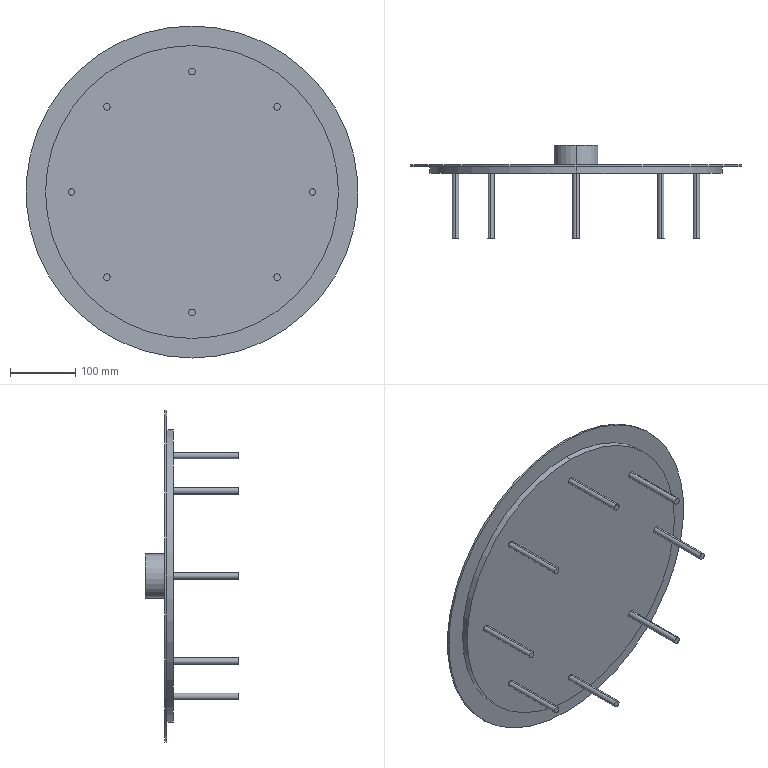Part | SolidWorks | features ICE 3, Extrusion 1 | 1 solid | 34 faces | box 510 x 143 x 510 mm | volume 2374097 mm3 | cylinder 22 | plane 12 | commonest cylinder face diameters 10 x16 67.699 x2 450 x2 510 x2
STEP:
#1=CARTESIAN_POINT('',(0.,43.,33.849));
#2=VERTEX_POINT('',#1);
#3=CARTESIAN_POINT('',(0.,43.,-33.849));
#4=VERTEX_POINT('',#3);
#5=CARTESIAN_POINT('',(0.,43.,0.));
#6=DIRECTION('',(0.,1.,0.));
#7=DIRECTION('',(0.,0.,1.));
#8=AXIS2_PLACEMENT_3D('',#5,#6,#7);
#9=CIRCLE('',#8,33.849);
#10=EDGE_CURVE('',#2,#4,#9,.T.);
#11=ORIENTED_EDGE('',*,*,#10,.F.);
#12=CARTESIAN_POINT('',(0.,13.,33.849));
#13=VERTEX_POINT('',#12);
#14=CARTESIAN_POINT('',(0.,43.,33.849));
#15=DIRECTION('',(0.,-1.,0.));
#16=VECTOR('',#15,1000.);
#17=LINE('',#14,#16);
#18=EDGE_CURVE('',#2,#13,#17,.T.);
#19=ORIENTED_EDGE('',*,*,#18,.T.);
#20=CARTESIAN_POINT('',(0.,13.,-33.849));
#21=VERTEX_POINT('',#20);
#22=CARTESIAN_POINT('',(0.,13.,0.));
#23=DIRECTION('',(0.,1.,0.));
#24=DIRECTION('',(0.,0.,1.));
#25=AXIS2_PLACEMENT_3D('',#22,#23,#24);
#26=CIRCLE('',#25,33.849);
#27=EDGE_CURVE('',#13,#21,#26,.T.);
#28=ORIENTED_EDGE('',*,*,#27,.T.);
#29=CARTESIAN_POINT('',(0.,43.,-33.849));
#30=DIRECTION('',(0.,-1.,0.));
#31=VECTOR('',#30,1000.);
#32=LINE('',#29,#31);
#33=EDGE_CURVE('',#4,#21,#32,.T.);
#34=ORIENTED_EDGE('',*,*,#33,.F.);
#35=EDGE_LOOP('',(#11,#19,#28,#34));
#36=FACE_OUTER_BOUND('',#35,.T.);
#37=CARTESIAN_POINT('',(0.,43.,0.));
#38=DIRECTION('',(0.,-1.,0.));
#39=DIRECTION('',(0.,0.,-1.));
#40=AXIS2_PLACEMENT_3D('',#37,#38,#39);
#41=CYLINDRICAL_SURFACE('',#40,33.849);
#42=ADVANCED_FACE('',(#36),#41,.T.);
#43=CARTESIAN_POINT('',(0.,13.,255.));
#44=VERTEX_POINT('',#43);
#45=CARTESIAN_POINT('',(0.,13.,-255.));
#46=VERTEX_POINT('',#45);
#47=CARTESIAN_POINT('',(0.,13.,0.));
#48=DIRECTION('',(0.,1.,0.));
#49=DIRECTION('',(0.,0.,1.));
#50=AXIS2_PLACEMENT_3D('',#47,#48,#49);
#51=CIRCLE('',#50,255.);
#52=EDGE_CURVE('',#44,#46,#51,.T.);
#53=ORIENTED_EDGE('',*,*,#52,.F.);
#54=CARTESIAN_POINT('',(0.,10.,255.));
#55=VERTEX_POINT('',#54);
#56=CARTESIAN_POINT('',(0.,13.,255.));
#57=DIRECTION('',(0.,-1.,0.));
#58=VECTOR('',#57,1000.);
#59=LINE('',#56,#58);
#60=EDGE_CURVE('',#44,#55,#59,.T.);
#61=ORIENTED_EDGE('',*,*,#60,.T.);
#62=CARTESIAN_POINT('',(0.,10.,-255.));
#63=VERTEX_POINT('',#62);
#64=CARTESIAN_POINT('',(0.,10.,0.));
#65=DIRECTION('',(0.,1.,0.));
#66=DIRECTION('',(0.,0.,1.));
#67=AXIS2_PLACEMENT_3D('',#64,#65,#66);
#68=CIRCLE('',#67,255.);
#69=EDGE_CURVE('',#55,#63,#68,.T.);
#70=ORIENTED_EDGE('',*,*,#69,.T.);
#71=CARTESIAN_POINT('',(0.,13.,-255.));
#72=DIRECTION('',(0.,-1.,0.));
#73=VECTOR('',#72,1000.);
#74=LINE('',#71,#73);
#75=EDGE_CURVE('',#46,#63,#74,.T.);
#76=ORIENTED_EDGE('',*,*,#75,.F.);
#77=EDGE_LOOP('',(#53,#61,#70,#76));
#78=FACE_OUTER_BOUND('',#77,.T.);
#79=CARTESIAN_POINT('',(0.,13.,0.));
#80=DIRECTION('',(0.,-1.,0.));
#81=DIRECTION('',(0.,0.,-1.));
#82=AXIS2_PLACEMENT_3D('',#79,#80,#81);
#83=CYLINDRICAL_SURFACE('',#82,255.);
#84=ADVANCED_FACE('',(#78),#83,.T.);
#85=CARTESIAN_POINT('',(-130.815,-100.,-135.815));
#86=VERTEX_POINT('',#85);
#87=CARTESIAN_POINT('',(-130.815,-100.,-125.815));
#88=VERTEX_POINT('',#87);
#89=CARTESIAN_POINT('',(-130.815,-100.,-130.815));
#90=DIRECTION('',(0.,-1.,0.));
#91=DIRECTION('',(0.,0.,-1.));
#92=AXIS2_PLACEMENT_3D('',#89,#90,#91);
#93=CIRCLE('',#92,5.);
#94=EDGE_CURVE('',#86,#88,#93,.T.);
#95=ORIENTED_EDGE('',*,*,#94,.F.);
#96=CARTESIAN_POINT('',(-130.815,0.,-135.815));
#97=VERTEX_POINT('',#96);
#98=CARTESIAN_POINT('',(-130.815,-100.,-135.815));
#99=DIRECTION('',(0.,1.,0.));
#100=VECTOR('',#99,1000.);
#101=LINE('',#98,#100);
#102=EDGE_CURVE('',#86,#97,#101,.T.);
#103=ORIENTED_EDGE('',*,*,#102,.T.);
#104=CARTESIAN_POINT('',(-130.815,0.,-125.815));
#105=VERTEX_POINT('',#104);
#106=CARTESIAN_POINT('',(-130.815,0.,-130.815));
#107=DIRECTION('',(0.,-1.,0.));
#108=DIRECTION('',(0.,0.,1.));
#109=AXIS2_PLACEMENT_3D('',#106,#107,#108);
#110=CIRCLE('',#109,5.);
#111=EDGE_CURVE('',#97,#105,#110,.T.);
#112=ORIENTED_EDGE('',*,*,#111,.T.);
#113=CARTESIAN_POINT('',(-130.815,-100.,-125.815));
#114=DIRECTION('',(0.,1.,0.));
#115=VECTOR('',#114,1000.);
#116=LINE('',#113,#115);
#117=EDGE_CURVE('',#88,#105,#116,.T.);
#118=ORIENTED_EDGE('',*,*,#117,.F.);
#119=EDGE_LOOP('',(#95,#103,#112,#118));
#120=FACE_OUTER_BOUND('',#119,.T.);
#121=CARTESIAN_POINT('',(-130.815,-100.,-130.815));
#122=DIRECTION('',(0.,1.,0.));
#123=DIRECTION('',(0.,0.,1.));
#124=AXIS2_PLACEMENT_3D('',#121,#122,#123);
#125=CYLINDRICAL_SURFACE('',#124,5.);
#126=ADVANCED_FACE('',(#120),#125,.T.);
#127=CARTESIAN_POINT('',(0.,-100.,-190.));
#128=VERTEX_POINT('',#127);
#129=CARTESIAN_POINT('',(0.,-100.,-180.));
#130=VERTEX_POINT('',#129);
#131=CARTESIAN_POINT('',(0.,-100.,-185.));
#132=DIRECTION('',(0.,-1.,0.));
#133=DIRECTION('',(0.,0.,-1.));
#134=AXIS2_PLACEMENT_3D('',#131,#132,#133);
#135=CIRCLE('',#134,5.);
#136=EDGE_CURVE('',#128,#130,#135,.T.);
#137=ORIENTED_EDGE('',*,*,#136,.F.);
#138=CARTESIAN_POINT('',(0.,0.,-190.));
#139=VERTEX_POINT('',#138);
#140=CARTESIAN_POINT('',(0.,-100.,-190.));
#141=DIRECTION('',(0.,1.,0.));
#142=VECTOR('',#141,1000.);
#143=LINE('',#140,#142);
#144=EDGE_CURVE('',#128,#139,#143,.T.);
#145=ORIENTED_EDGE('',*,*,#144,.T.);
#146=CARTESIAN_POINT('',(0.,0.,-180.));
#147=VERTEX_POINT('',#146);
#148=CARTESIAN_POINT('',(0.,0.,-185.));
#149=DIRECTION('',(0.,-1.,0.));
#150=DIRECTION('',(0.,0.,1.));
#151=AXIS2_PLACEMENT_3D('',#148,#149,#150);
#152=CIRCLE('',#151,5.);
#153=EDGE_CURVE('',#139,#147,#152,.T.);
#154=ORIENTED_EDGE('',*,*,#153,.T.);
#155=CARTESIAN_POINT('',(0.,-100.,-180.));
#156=DIRECTION('',(0.,1.,0.));
#157=VECTOR('',#156,1000.);
#158=LINE('',#155,#157);
#159=EDGE_CURVE('',#130,#147,#158,.T.);
#160=ORIENTED_EDGE('',*,*,#159,.F.);
#161=EDGE_LOOP('',(#137,#145,#154,#160));
#162=FACE_OUTER_BOUND('',#161,.T.);
#163=CARTESIAN_POINT('',(0.,-100.,-185.));
#164=DIRECTION('',(0.,1.,0.));
#165=DIRECTION('',(0.,0.,1.));
#166=AXIS2_PLACEMENT_3D('',#163,#164,#165);
#167=CYLINDRICAL_SURFACE('',#166,5.);
#168=ADVANCED_FACE('',(#162),#167,.T.);
#169=CARTESIAN_POINT('',(130.815,-100.,-135.815));
#170=VERTEX_POINT('',#169);
#171=CARTESIAN_POINT('',(130.815,-100.,-125.815));
#172=VERTEX_POINT('',#171);
#173=CARTESIAN_POINT('',(130.815,-100.,-130.815));
#174=DIRECTION('',(0.,-1.,0.));
#175=DIRECTION('',(0.,0.,-1.));
#176=AXIS2_PLACEMENT_3D('',#173,#174,#175);
#177=CIRCLE('',#176,5.);
#178=EDGE_CURVE('',#170,#172,#177,.T.);
#179=ORIENTED_EDGE('',*,*,#178,.F.);
#180=CARTESIAN_POINT('',(130.815,0.,-135.815));
#181=VERTEX_POINT('',#180);
#182=CARTESIAN_POINT('',(130.815,-100.,-135.815));
#183=DIRECTION('',(0.,1.,0.));
#184=VECTOR('',#183,1000.);
#185=LINE('',#182,#184);
#186=EDGE_CURVE('',#170,#181,#185,.T.);
#187=ORIENTED_EDGE('',*,*,#186,.T.);
#188=CARTESIAN_POINT('',(130.815,0.,-125.815));
#189=VERTEX_POINT('',#188);
#190=CARTESIAN_POINT('',(130.815,0.,-130.815));
#191=DIRECTION('',(0.,-1.,0.));
#192=DIRECTION('',(0.,0.,1.));
#193=AXIS2_PLACEMENT_3D('',#190,#191,#192);
#194=CIRCLE('',#193,5.);
#195=EDGE_CURVE('',#181,#189,#194,.T.);
#196=ORIENTED_EDGE('',*,*,#195,.T.);
#197=CARTESIAN_POINT('',(130.815,-100.,-125.815));
#198=DIRECTION('',(0.,1.,0.));
#199=VECTOR('',#198,1000.);
#200=LINE('',#197,#199);
#201=EDGE_CURVE('',#172,#189,#200,.T.);
#202=ORIENTED_EDGE('',*,*,#201,.F.);
#203=EDGE_LOOP('',(#179,#187,#196,#202));
#204=FACE_OUTER_BOUND('',#203,.T.);
#205=CARTESIAN_POINT('',(130.815,-100.,-130.815));
#206=DIRECTION('',(0.,1.,0.));
#207=DIRECTION('',(0.,0.,1.));
#208=AXIS2_PLACEMENT_3D('',#205,#206,#207);
#209=CYLINDRICAL_SURFACE('',#208,5.);
#210=ADVANCED_FACE('',(#204),#209,.T.);
#211=CARTESIAN_POINT('',(185.,-100.,-5.));
#212=VERTEX_POINT('',#211);
#213=CARTESIAN_POINT('',(185.,-100.,5.));
#214=VERTEX_POINT('',#213);
#215=CARTESIAN_POINT('',(185.,-100.,0.));
#216=DIRECTION('',(0.,-1.,0.));
#217=DIRECTION('',(0.,0.,-1.));
#218=AXIS2_PLACEMENT_3D('',#215,#216,#217);
#219=CIRCLE('',#218,5.);
#220=EDGE_CURVE('',#212,#214,#219,.T.);
#221=ORIENTED_EDGE('',*,*,#220,.F.);
#222=CARTESIAN_POINT('',(185.,0.,-5.));
#223=VERTEX_POINT('',#222);
#224=CARTESIAN_POINT('',(185.,-100.,-5.));
#225=DIRECTION('',(0.,1.,0.));
#226=VECTOR('',#225,1000.);
#227=LINE('',#224,#226);
#228=EDGE_CURVE('',#212,#223,#227,.T.);
#229=ORIENTED_EDGE('',*,*,#228,.T.);
#230=CARTESIAN_POINT('',(185.,0.,5.));
#231=VERTEX_POINT('',#230);
#232=CARTESIAN_POINT('',(185.,0.,0.));
#233=DIRECTION('',(0.,-1.,0.));
#234=DIRECTION('',(0.,0.,1.));
#235=AXIS2_PLACEMENT_3D('',#232,#233,#234);
#236=CIRCLE('',#235,5.);
#237=EDGE_CURVE('',#223,#231,#236,.T.);
#238=ORIENTED_EDGE('',*,*,#237,.T.);
#239=CARTESIAN_POINT('',(185.,-100.,5.));
#240=DIRECTION('',(0.,1.,0.));
#241=VECTOR('',#240,1000.);
#242=LINE('',#239,#241);
#243=EDGE_CURVE('',#214,#231,#242,.T.);
#244=ORIENTED_EDGE('',*,*,#243,.F.);
#245=EDGE_LOOP('',(#221,#229,#238,#244));
#246=FACE_OUTER_BOUND('',#245,.T.);
#247=CARTESIAN_POINT('',(185.,-100.,0.));
#248=DIRECTION('',(0.,1.,0.));
#249=DIRECTION('',(0.,0.,1.));
#250=AXIS2_PLACEMENT_3D('',#247,#248,#249);
#251=CYLINDRICAL_SURFACE('',#250,5.);
#252=ADVANCED_FACE('',(#246),#251,.T.);
#253=CARTESIAN_POINT('',(130.815,-100.,125.815));
#254=VERTEX_POINT('',#253);
#255=CARTESIAN_POINT('',(130.815,-100.,135.815));
#256=VERTEX_POINT('',#255);
#257=CARTESIAN_POINT('',(130.815,-100.,130.815));
#258=DIRECTION('',(0.,-1.,0.));
#259=DIRECTION('',(0.,0.,-1.));
#260=AXIS2_PLACEMENT_3D('',#257,#258,#259);
#261=CIRCLE('',#260,5.);
#262=EDGE_CURVE('',#254,#256,#261,.T.);
#263=ORIENTED_EDGE('',*,*,#262,.F.);
#264=CARTESIAN_POINT('',(130.815,0.,125.815));
#265=VERTEX_POINT('',#264);
#266=CARTESIAN_POINT('',(130.815,-100.,125.815));
#267=DIRECTION('',(0.,1.,0.));
#268=VECTOR('',#267,1000.);
#269=LINE('',#266,#268);
#270=EDGE_CURVE('',#254,#265,#269,.T.);
#271=ORIENTED_EDGE('',*,*,#270,.T.);
#272=CARTESIAN_POINT('',(130.815,0.,135.815));
#273=VERTEX_POINT('',#272);
#274=CARTESIAN_POINT('',(130.815,0.,130.815));
#275=DIRECTION('',(0.,-1.,0.));
#276=DIRECTION('',(0.,0.,1.));
#277=AXIS2_PLACEMENT_3D('',#274,#275,#276);
#278=CIRCLE('',#277,5.);
#279=EDGE_CURVE('',#265,#273,#278,.T.);
#280=ORIENTED_EDGE('',*,*,#279,.T.);
#281=CARTESIAN_POINT('',(130.815,-100.,135.815));
#282=DIRECTION('',(0.,1.,0.));
#283=VECTOR('',#282,1000.);
#284=LINE('',#281,#283);
#285=EDGE_CURVE('',#256,#273,#284,.T.);
#286=ORIENTED_EDGE('',*,*,#285,.F.);
#287=EDGE_LOOP('',(#263,#271,#280,#286));
#288=FACE_OUTER_BOUND('',#287,.T.);
#289=CARTESIAN_POINT('',(130.815,-100.,130.815));
#290=DIRECTION('',(0.,1.,0.));
#291=DIRECTION('',(0.,0.,1.));
#292=AXIS2_PLACEMENT_3D('',#289,#290,#291);
#293=CYLINDRICAL_SURFACE('',#292,5.);
#294=ADVANCED_FACE('',(#288),#293,.T.);
#295=CARTESIAN_POINT('',(0.,-100.,180.));
#296=VERTEX_POINT('',#295);
#297=CARTESIAN_POINT('',(0.,-100.,190.));
#298=VERTEX_POINT('',#297);
#299=CARTESIAN_POINT('',(0.,-100.,185.));
#300=DIRECTION('',(0.,-1.,0.));
#301=DIRECTION('',(0.,0.,-1.));
#302=AXIS2_PLACEMENT_3D('',#299,#300,#301);
#303=CIRCLE('',#302,5.);
#304=EDGE_CURVE('',#296,#298,#303,.T.);
#305=ORIENTED_EDGE('',*,*,#304,.F.);
#306=CARTESIAN_POINT('',(0.,0.,180.));
#307=VERTEX_POINT('',#306);
#308=CARTESIAN_POINT('',(0.,-100.,180.));
#309=DIRECTION('',(0.,1.,0.));
#310=VECTOR('',#309,1000.);
#311=LINE('',#308,#310);
#312=EDGE_CURVE('',#296,#307,#311,.T.);
#313=ORIENTED_EDGE('',*,*,#312,.T.);
#314=CARTESIAN_POINT('',(0.,0.,190.));
#315=VERTEX_POINT('',#314);
#316=CARTESIAN_POINT('',(0.,0.,185.));
#317=DIRECTION('',(0.,-1.,0.));
#318=DIRECTION('',(0.,0.,1.));
#319=AXIS2_PLACEMENT_3D('',#316,#317,#318);
#320=CIRCLE('',#319,5.);
#321=EDGE_CURVE('',#307,#315,#320,.T.);
#322=ORIENTED_EDGE('',*,*,#321,.T.);
#323=CARTESIAN_POINT('',(0.,-100.,190.));
#324=DIRECTION('',(0.,1.,0.));
#325=VECTOR('',#324,1000.);
#326=LINE('',#323,#325);
#327=EDGE_CURVE('',#298,#315,#326,.T.);
#328=ORIENTED_EDGE('',*,*,#327,.F.);
#329=EDGE_LOOP('',(#305,#313,#322,#328));
#330=FACE_OUTER_BOUND('',#329,.T.);
#331=CARTESIAN_POINT('',(0.,-100.,185.));
#332=DIRECTION('',(0.,1.,0.));
#333=DIRECTION('',(0.,0.,1.));
#334=AXIS2_PLACEMENT_3D('',#331,#332,#333);
#335=CYLINDRICAL_SURFACE('',#334,5.);
#336=ADVANCED_FACE('',(#330),#335,.T.);
#337=CARTESIAN_POINT('',(-130.815,-100.,125.815));
#338=VERTEX_POINT('',#337);
#339=CARTESIAN_POINT('',(-130.815,-100.,135.815));
#340=VERTEX_POINT('',#339);
#341=CARTESIAN_POINT('',(-130.815,-100.,130.815));
#342=DIRECTION('',(0.,-1.,0.));
#343=DIRECTION('',(0.,0.,-1.));
#344=AXIS2_PLACEMENT_3D('',#341,#342,#343);
#345=CIRCLE('',#344,5.);
#346=EDGE_CURVE('',#338,#340,#345,.T.);
#347=ORIENTED_EDGE('',*,*,#346,.F.);
#348=CARTESIAN_POINT('',(-130.815,0.,125.815));
#349=VERTEX_POINT('',#348);
#350=CARTESIAN_POINT('',(-130.815,-100.,125.815));
#351=DIRECTION('',(0.,1.,0.));
#352=VECTOR('',#351,1000.);
#353=LINE('',#350,#352);
#354=EDGE_CURVE('',#338,#349,#353,.T.);
#355=ORIENTED_EDGE('',*,*,#354,.T.);
#356=CARTESIAN_POINT('',(-130.815,0.,135.815));
#357=VERTEX_POINT('',#356);
#358=CARTESIAN_POINT('',(-130.815,0.,130.815));
#359=DIRECTION('',(0.,-1.,0.));
#360=DIRECTION('',(0.,0.,1.));
#361=AXIS2_PLACEMENT_3D('',#358,#359,#360);
#362=CIRCLE('',#361,5.);
#363=EDGE_CURVE('',#349,#357,#362,.T.);
#364=ORIENTED_EDGE('',*,*,#363,.T.);
#365=CARTESIAN_POINT('',(-130.815,-100.,135.815));
#366=DIRECTION('',(0.,1.,0.));
#367=VECTOR('',#366,1000.);
#368=LINE('',#365,#367);
#369=EDGE_CURVE('',#340,#357,#368,.T.);
#370=ORIENTED_EDGE('',*,*,#369,.F.);
#371=EDGE_LOOP('',(#347,#355,#364,#370));
#372=FACE_OUTER_BOUND('',#371,.T.);
#373=CARTESIAN_POINT('',(-130.815,-100.,130.815));
#374=DIRECTION('',(0.,1.,0.));
#375=DIRECTION('',(0.,0.,1.));
#376=AXIS2_PLACEMENT_3D('',#373,#374,#375);
#377=CYLINDRICAL_SURFACE('',#376,5.);
#378=ADVANCED_FACE('',(#372),#377,.T.);
#379=CARTESIAN_POINT('',(-185.,-100.,-5.));
#380=VERTEX_POINT('',#379);
#381=CARTESIAN_POINT('',(-185.,-100.,5.));
#382=VERTEX_POINT('',#381);
#383=CARTESIAN_POINT('',(-185.,-100.,0.));
#384=DIRECTION('',(0.,-1.,0.));
#385=DIRECTION('',(0.,0.,-1.));
#386=AXIS2_PLACEMENT_3D('',#383,#384,#385);
#387=CIRCLE('',#386,5.);
#388=EDGE_CURVE('',#380,#382,#387,.T.);
#389=ORIENTED_EDGE('',*,*,#388,.F.);
#390=CARTESIAN_POINT('',(-185.,0.,-5.));
#391=VERTEX_POINT('',#390);
#392=CARTESIAN_POINT('',(-185.,-100.,-5.));
#393=DIRECTION('',(0.,1.,0.));
#394=VECTOR('',#393,1000.);
#395=LINE('',#392,#394);
#396=EDGE_CURVE('',#380,#391,#395,.T.);
#397=ORIENTED_EDGE('',*,*,#396,.T.);
#398=CARTESIAN_POINT('',(-185.,0.,5.));
#399=VERTEX_POINT('',#398);
#400=CARTESIAN_POINT('',(-185.,0.,0.));
#401=DIRECTION('',(0.,-1.,0.));
#402=DIRECTION('',(0.,0.,1.));
#403=AXIS2_PLACEMENT_3D('',#400,#401,#402);
#404=CIRCLE('',#403,5.);
#405=EDGE_CURVE('',#391,#399,#404,.T.);
#406=ORIENTED_EDGE('',*,*,#405,.T.);
#407=CARTESIAN_POINT('',(-185.,-100.,5.));
#408=DIRECTION('',(0.,1.,0.));
#409=VECTOR('',#408,1000.);
#410=LINE('',#407,#409);
#411=EDGE_CURVE('',#382,#399,#410,.T.);
#412=ORIENTED_EDGE('',*,*,#411,.F.);
#413=EDGE_LOOP('',(#389,#397,#406,#412));
#414=FACE_OUTER_BOUND('',#413,.T.);
#415=CARTESIAN_POINT('',(-185.,-100.,0.));
#416=DIRECTION('',(0.,1.,0.));
#417=DIRECTION('',(0.,0.,1.));
#418=AXIS2_PLACEMENT_3D('',#415,#416,#417);
#419=CYLINDRICAL_SURFACE('',#418,5.);
#420=ADVANCED_FACE('',(#414),#419,.T.);
#421=CARTESIAN_POINT('',(0.,10.,225.));
#422=VERTEX_POINT('',#421);
#423=CARTESIAN_POINT('',(0.,10.,-225.));
#424=VERTEX_POINT('',#423);
#425=CARTESIAN_POINT('',(0.,10.,0.));
#426=DIRECTION('',(0.,1.,0.));
#427=DIRECTION('',(0.,0.,1.));
#428=AXIS2_PLACEMENT_3D('',#425,#426,#427);
#429=CIRCLE('',#428,225.);
#430=EDGE_CURVE('',#422,#424,#429,.T.);
#431=ORIENTED_EDGE('',*,*,#430,.F.);
#432=CARTESIAN_POINT('',(0.,0.,225.));
#433=VERTEX_POINT('',#432);
#434=CARTESIAN_POINT('',(0.,10.,225.));
#435=DIRECTION('',(0.,-1.,0.));
#436=VECTOR('',#435,1000.);
#437=LINE('',#434,#436);
#438=EDGE_CURVE('',#422,#433,#437,.T.);
#439=ORIENTED_EDGE('',*,*,#438,.T.);
#440=CARTESIAN_POINT('',(0.,0.,-225.));
#441=VERTEX_POINT('',#440);
#442=CARTESIAN_POINT('',(0.,0.,0.));
#443=DIRECTION('',(0.,1.,0.));
#444=DIRECTION('',(0.,0.,1.));
#445=AXIS2_PLACEMENT_3D('',#442,#443,#444);
#446=CIRCLE('',#445,225.);
#447=EDGE_CURVE('',#433,#441,#446,.T.);
#448=ORIENTED_EDGE('',*,*,#447,.T.);
#449=CARTESIAN_POINT('',(0.,10.,-225.));
#450=DIRECTION('',(0.,-1.,0.));
#451=VECTOR('',#450,1000.);
#452=LINE('',#449,#451);
#453=EDGE_CURVE('',#424,#441,#452,.T.);
#454=ORIENTED_EDGE('',*,*,#453,.F.);
#455=EDGE_LOOP('',(#431,#439,#448,#454));
#456=FACE_OUTER_BOUND('',#455,.T.);
#457=CARTESIAN_POINT('',(0.,10.,0.));
#458=DIRECTION('',(0.,-1.,0.));
#459=DIRECTION('',(0.,0.,-1.));
#460=AXIS2_PLACEMENT_3D('',#457,#458,#459);
#461=CYLINDRICAL_SURFACE('',#460,225.);
#462=ADVANCED_FACE('',(#456),#461,.T.);
#463=ORIENTED_EDGE('',*,*,#438,.F.);
#464=CARTESIAN_POINT('',(0.,10.,0.));
#465=DIRECTION('',(0.,1.,0.));
#466=DIRECTION('',(0.,0.,1.));
#467=AXIS2_PLACEMENT_3D('',#464,#465,#466);
#468=CIRCLE('',#467,225.);
#469=EDGE_CURVE('',#424,#422,#468,.T.);
#470=ORIENTED_EDGE('',*,*,#469,.F.);
#471=ORIENTED_EDGE('',*,*,#453,.T.);
#472=CARTESIAN_POINT('',(0.,0.,0.));
#473=DIRECTION('',(0.,1.,0.));
#474=DIRECTION('',(0.,0.,1.));
#475=AXIS2_PLACEMENT_3D('',#472,#473,#474);
#476=CIRCLE('',#475,225.);
#477=EDGE_CURVE('',#441,#433,#476,.T.);
#478=ORIENTED_EDGE('',*,*,#477,.T.);
#479=EDGE_LOOP('',(#463,#470,#471,#478));
#480=FACE_OUTER_BOUND('',#479,.T.);
#481=CARTESIAN_POINT('',(0.,10.,0.));
#482=DIRECTION('',(0.,-1.,0.));
#483=DIRECTION('',(0.,0.,-1.));
#484=AXIS2_PLACEMENT_3D('',#481,#482,#483);
#485=CYLINDRICAL_SURFACE('',#484,225.);
#486=ADVANCED_FACE('',(#480),#485,.T.);
#487=CARTESIAN_POINT('',(-130.815,0.,-130.815));
#488=DIRECTION('',(0.,-1.,0.));
#489=DIRECTION('',(0.,0.,1.));
#490=AXIS2_PLACEMENT_3D('',#487,#488,#489);
#491=CIRCLE('',#490,5.);
#492=EDGE_CURVE('',#105,#97,#491,.T.);
#493=ORIENTED_EDGE('',*,*,#492,.F.);
#494=ORIENTED_EDGE('',*,*,#111,.F.);
#495=EDGE_LOOP('',(#493,#494));
#496=FACE_BOUND('',#495,.T.);
#497=CARTESIAN_POINT('',(0.,0.,-185.));
#498=DIRECTION('',(0.,-1.,0.));
#499=DIRECTION('',(0.,0.,1.));
#500=AXIS2_PLACEMENT_3D('',#497,#498,#499);
#501=CIRCLE('',#500,5.);
#502=EDGE_CURVE('',#147,#139,#501,.T.);
#503=ORIENTED_EDGE('',*,*,#502,.F.);
#504=ORIENTED_EDGE('',*,*,#153,.F.);
#505=EDGE_LOOP('',(#503,#504));
#506=FACE_BOUND('',#505,.T.);
#507=CARTESIAN_POINT('',(130.815,0.,-130.815));
#508=DIRECTION('',(0.,-1.,0.));
#509=DIRECTION('',(0.,0.,1.));
#510=AXIS2_PLACEMENT_3D('',#507,#508,#509);
#511=CIRCLE('',#510,5.);
#512=EDGE_CURVE('',#189,#181,#511,.T.);
#513=ORIENTED_EDGE('',*,*,#512,.F.);
#514=ORIENTED_EDGE('',*,*,#195,.F.);
#515=EDGE_LOOP('',(#513,#514));
#516=FACE_BOUND('',#515,.T.);
#517=CARTESIAN_POINT('',(185.,0.,0.));
#518=DIRECTION('',(0.,-1.,0.));
#519=DIRECTION('',(0.,0.,1.));
#520=AXIS2_PLACEMENT_3D('',#517,#518,#519);
#521=CIRCLE('',#520,5.);
#522=EDGE_CURVE('',#231,#223,#521,.T.);
#523=ORIENTED_EDGE('',*,*,#522,.F.);
#524=ORIENTED_EDGE('',*,*,#237,.F.);
#525=EDGE_LOOP('',(#523,#524));
#526=FACE_BOUND('',#525,.T.);
#527=CARTESIAN_POINT('',(130.815,0.,130.815));
#528=DIRECTION('',(0.,-1.,0.));
#529=DIRECTION('',(0.,0.,1.));
#530=AXIS2_PLACEMENT_3D('',#527,#528,#529);
#531=CIRCLE('',#530,5.);
#532=EDGE_CURVE('',#273,#265,#531,.T.);
#533=ORIENTED_EDGE('',*,*,#532,.F.);
#534=ORIENTED_EDGE('',*,*,#279,.F.);
#535=EDGE_LOOP('',(#533,#534));
#536=FACE_BOUND('',#535,.T.);
#537=CARTESIAN_POINT('',(0.,0.,185.));
#538=DIRECTION('',(0.,-1.,0.));
#539=DIRECTION('',(0.,0.,1.));
#540=AXIS2_PLACEMENT_3D('',#537,#538,#539);
#541=CIRCLE('',#540,5.);
#542=EDGE_CURVE('',#315,#307,#541,.T.);
#543=ORIENTED_EDGE('',*,*,#542,.F.);
#544=ORIENTED_EDGE('',*,*,#321,.F.);
#545=EDGE_LOOP('',(#543,#544));
#546=FACE_BOUND('',#545,.T.);
#547=CARTESIAN_POINT('',(-130.815,0.,130.815));
#548=DIRECTION('',(0.,-1.,0.));
#549=DIRECTION('',(0.,0.,1.));
#550=AXIS2_PLACEMENT_3D('',#547,#548,#549);
#551=CIRCLE('',#550,5.);
#552=EDGE_CURVE('',#357,#349,#551,.T.);
#553=ORIENTED_EDGE('',*,*,#552,.F.);
#554=ORIENTED_EDGE('',*,*,#363,.F.);
#555=EDGE_LOOP('',(#553,#554));
#556=FACE_BOUND('',#555,.T.);
#557=CARTESIAN_POINT('',(-185.,0.,0.));
#558=DIRECTION('',(0.,-1.,0.));
#559=DIRECTION('',(0.,0.,1.));
#560=AXIS2_PLACEMENT_3D('',#557,#558,#559);
#561=CIRCLE('',#560,5.);
#562=EDGE_CURVE('',#399,#391,#561,.T.);
#563=ORIENTED_EDGE('',*,*,#562,.F.);
#564=ORIENTED_EDGE('',*,*,#405,.F.);
#565=EDGE_LOOP('',(#563,#564));
#566=FACE_BOUND('',#565,.T.);
#567=ORIENTED_EDGE('',*,*,#477,.F.);
#568=ORIENTED_EDGE('',*,*,#447,.F.);
#569=EDGE_LOOP('',(#567,#568));
#570=FACE_OUTER_BOUND('',#569,.T.);
#571=CARTESIAN_POINT('',(0.,0.,0.));
#572=DIRECTION('',(0.,1.,0.));
#573=DIRECTION('',(0.,0.,1.));
#574=AXIS2_PLACEMENT_3D('',#571,#572,#573);
#575=PLANE('',#574);
#576=ADVANCED_FACE('',(#496,#506,#516,#526,#536,#546,#556,#566,#570),#575,.F.);
#577=ORIENTED_EDGE('',*,*,#396,.F.);
#578=CARTESIAN_POINT('',(-185.,-100.,0.));
#579=DIRECTION('',(0.,-1.,0.));
#580=DIRECTION('',(0.,0.,-1.));
#581=AXIS2_PLACEMENT_3D('',#578,#579,#580);
#582=CIRCLE('',#581,5.);
#583=EDGE_CURVE('',#382,#380,#582,.T.);
#584=ORIENTED_EDGE('',*,*,#583,.F.);
#585=ORIENTED_EDGE('',*,*,#411,.T.);
#586=ORIENTED_EDGE('',*,*,#562,.T.);
#587=EDGE_LOOP('',(#577,#584,#585,#586));
#588=FACE_OUTER_BOUND('',#587,.T.);
#589=CARTESIAN_POINT('',(-185.,-100.,0.));
#590=DIRECTION('',(0.,1.,0.));
#591=DIRECTION('',(0.,0.,1.));
#592=AXIS2_PLACEMENT_3D('',#589,#590,#591);
#593=CYLINDRICAL_SURFACE('',#592,5.);
#594=ADVANCED_FACE('',(#588),#593,.T.);
#595=ORIENTED_EDGE('',*,*,#583,.T.);
#596=ORIENTED_EDGE('',*,*,#388,.T.);
#597=EDGE_LOOP('',(#595,#596));
#598=FACE_OUTER_BOUND('',#597,.T.);
#599=CARTESIAN_POINT('',(-185.,-100.,0.));
#600=DIRECTION('',(0.,-1.,0.));
#601=DIRECTION('',(0.,0.,-1.));
#602=AXIS2_PLACEMENT_3D('',#599,#600,#601);
#603=PLANE('',#602);
#604=ADVANCED_FACE('',(#598),#603,.T.);
#605=ORIENTED_EDGE('',*,*,#354,.F.);
#606=CARTESIAN_POINT('',(-130.815,-100.,130.815));
#607=DIRECTION('',(0.,-1.,0.));
#608=DIRECTION('',(0.,0.,-1.));
#609=AXIS2_PLACEMENT_3D('',#606,#607,#608);
#610=CIRCLE('',#609,5.);
#611=EDGE_CURVE('',#340,#338,#610,.T.);
#612=ORIENTED_EDGE('',*,*,#611,.F.);
#613=ORIENTED_EDGE('',*,*,#369,.T.);
#614=ORIENTED_EDGE('',*,*,#552,.T.);
#615=EDGE_LOOP('',(#605,#612,#613,#614));
#616=FACE_OUTER_BOUND('',#615,.T.);
#617=CARTESIAN_POINT('',(-130.815,-100.,130.815));
#618=DIRECTION('',(0.,1.,0.));
#619=DIRECTION('',(0.,0.,1.));
#620=AXIS2_PLACEMENT_3D('',#617,#618,#619);
#621=CYLINDRICAL_SURFACE('',#620,5.);
#622=ADVANCED_FACE('',(#616),#621,.T.);
#623=ORIENTED_EDGE('',*,*,#611,.T.);
#624=ORIENTED_EDGE('',*,*,#346,.T.);
#625=EDGE_LOOP('',(#623,#624));
#626=FACE_OUTER_BOUND('',#625,.T.);
#627=CARTESIAN_POINT('',(-130.815,-100.,130.815));
#628=DIRECTION('',(0.,-1.,0.));
#629=DIRECTION('',(0.,0.,-1.));
#630=AXIS2_PLACEMENT_3D('',#627,#628,#629);
#631=PLANE('',#630);
#632=ADVANCED_FACE('',(#626),#631,.T.);
#633=ORIENTED_EDGE('',*,*,#312,.F.);
#634=CARTESIAN_POINT('',(0.,-100.,185.));
#635=DIRECTION('',(0.,-1.,0.));
#636=DIRECTION('',(0.,0.,-1.));
#637=AXIS2_PLACEMENT_3D('',#634,#635,#636);
#638=CIRCLE('',#637,5.);
#639=EDGE_CURVE('',#298,#296,#638,.T.);
#640=ORIENTED_EDGE('',*,*,#639,.F.);
#641=ORIENTED_EDGE('',*,*,#327,.T.);
#642=ORIENTED_EDGE('',*,*,#542,.T.);
#643=EDGE_LOOP('',(#633,#640,#641,#642));
#644=FACE_OUTER_BOUND('',#643,.T.);
#645=CARTESIAN_POINT('',(0.,-100.,185.));
#646=DIRECTION('',(0.,1.,0.));
#647=DIRECTION('',(0.,0.,1.));
#648=AXIS2_PLACEMENT_3D('',#645,#646,#647);
#649=CYLINDRICAL_SURFACE('',#648,5.);
#650=ADVANCED_FACE('',(#644),#649,.T.);
#651=ORIENTED_EDGE('',*,*,#639,.T.);
#652=ORIENTED_EDGE('',*,*,#304,.T.);
#653=EDGE_LOOP('',(#651,#652));
#654=FACE_OUTER_BOUND('',#653,.T.);
#655=CARTESIAN_POINT('',(0.,-100.,185.));
#656=DIRECTION('',(0.,-1.,0.));
#657=DIRECTION('',(0.,0.,-1.));
#658=AXIS2_PLACEMENT_3D('',#655,#656,#657);
#659=PLANE('',#658);
#660=ADVANCED_FACE('',(#654),#659,.T.);
#661=ORIENTED_EDGE('',*,*,#270,.F.);
#662=CARTESIAN_POINT('',(130.815,-100.,130.815));
#663=DIRECTION('',(0.,-1.,0.));
#664=DIRECTION('',(0.,0.,-1.));
#665=AXIS2_PLACEMENT_3D('',#662,#663,#664);
#666=CIRCLE('',#665,5.);
#667=EDGE_CURVE('',#256,#254,#666,.T.);
#668=ORIENTED_EDGE('',*,*,#667,.F.);
#669=ORIENTED_EDGE('',*,*,#285,.T.);
#670=ORIENTED_EDGE('',*,*,#532,.T.);
#671=EDGE_LOOP('',(#661,#668,#669,#670));
#672=FACE_OUTER_BOUND('',#671,.T.);
#673=CARTESIAN_POINT('',(130.815,-100.,130.815));
#674=DIRECTION('',(0.,1.,0.));
#675=DIRECTION('',(0.,0.,1.));
#676=AXIS2_PLACEMENT_3D('',#673,#674,#675);
#677=CYLINDRICAL_SURFACE('',#676,5.);
#678=ADVANCED_FACE('',(#672),#677,.T.);
#679=ORIENTED_EDGE('',*,*,#667,.T.);
#680=ORIENTED_EDGE('',*,*,#262,.T.);
#681=EDGE_LOOP('',(#679,#680));
#682=FACE_OUTER_BOUND('',#681,.T.);
#683=CARTESIAN_POINT('',(130.815,-100.,130.815));
#684=DIRECTION('',(0.,-1.,0.));
#685=DIRECTION('',(0.,0.,-1.));
#686=AXIS2_PLACEMENT_3D('',#683,#684,#685);
#687=PLANE('',#686);
#688=ADVANCED_FACE('',(#682),#687,.T.);
#689=ORIENTED_EDGE('',*,*,#228,.F.);
#690=CARTESIAN_POINT('',(185.,-100.,0.));
#691=DIRECTION('',(0.,-1.,0.));
#692=DIRECTION('',(0.,0.,-1.));
#693=AXIS2_PLACEMENT_3D('',#690,#691,#692);
#694=CIRCLE('',#693,5.);
#695=EDGE_CURVE('',#214,#212,#694,.T.);
#696=ORIENTED_EDGE('',*,*,#695,.F.);
#697=ORIENTED_EDGE('',*,*,#243,.T.);
#698=ORIENTED_EDGE('',*,*,#522,.T.);
#699=EDGE_LOOP('',(#689,#696,#697,#698));
#700=FACE_OUTER_BOUND('',#699,.T.);
#701=CARTESIAN_POINT('',(185.,-100.,0.));
#702=DIRECTION('',(0.,1.,0.));
#703=DIRECTION('',(0.,0.,1.));
#704=AXIS2_PLACEMENT_3D('',#701,#702,#703);
#705=CYLINDRICAL_SURFACE('',#704,5.);
#706=ADVANCED_FACE('',(#700),#705,.T.);
#707=ORIENTED_EDGE('',*,*,#695,.T.);
#708=ORIENTED_EDGE('',*,*,#220,.T.);
#709=EDGE_LOOP('',(#707,#708));
#710=FACE_OUTER_BOUND('',#709,.T.);
#711=CARTESIAN_POINT('',(185.,-100.,0.));
#712=DIRECTION('',(0.,-1.,0.));
#713=DIRECTION('',(0.,0.,-1.));
#714=AXIS2_PLACEMENT_3D('',#711,#712,#713);
#715=PLANE('',#714);
#716=ADVANCED_FACE('',(#710),#715,.T.);
#717=ORIENTED_EDGE('',*,*,#186,.F.);
#718=CARTESIAN_POINT('',(130.815,-100.,-130.815));
#719=DIRECTION('',(0.,-1.,0.));
#720=DIRECTION('',(0.,0.,-1.));
#721=AXIS2_PLACEMENT_3D('',#718,#719,#720);
#722=CIRCLE('',#721,5.);
#723=EDGE_CURVE('',#172,#170,#722,.T.);
#724=ORIENTED_EDGE('',*,*,#723,.F.);
#725=ORIENTED_EDGE('',*,*,#201,.T.);
#726=ORIENTED_EDGE('',*,*,#512,.T.);
#727=EDGE_LOOP('',(#717,#724,#725,#726));
#728=FACE_OUTER_BOUND('',#727,.T.);
#729=CARTESIAN_POINT('',(130.815,-100.,-130.815));
#730=DIRECTION('',(0.,1.,0.));
#731=DIRECTION('',(0.,0.,1.));
#732=AXIS2_PLACEMENT_3D('',#729,#730,#731);
#733=CYLINDRICAL_SURFACE('',#732,5.);
#734=ADVANCED_FACE('',(#728),#733,.T.);
#735=ORIENTED_EDGE('',*,*,#723,.T.);
#736=ORIENTED_EDGE('',*,*,#178,.T.);
#737=EDGE_LOOP('',(#735,#736));
#738=FACE_OUTER_BOUND('',#737,.T.);
#739=CARTESIAN_POINT('',(130.815,-100.,-130.815));
#740=DIRECTION('',(0.,-1.,0.));
#741=DIRECTION('',(0.,0.,-1.));
#742=AXIS2_PLACEMENT_3D('',#739,#740,#741);
#743=PLANE('',#742);
#744=ADVANCED_FACE('',(#738),#743,.T.);
#745=ORIENTED_EDGE('',*,*,#144,.F.);
#746=CARTESIAN_POINT('',(0.,-100.,-185.));
#747=DIRECTION('',(0.,-1.,0.));
#748=DIRECTION('',(0.,0.,-1.));
#749=AXIS2_PLACEMENT_3D('',#746,#747,#748);
#750=CIRCLE('',#749,5.);
#751=EDGE_CURVE('',#130,#128,#750,.T.);
#752=ORIENTED_EDGE('',*,*,#751,.F.);
#753=ORIENTED_EDGE('',*,*,#159,.T.);
#754=ORIENTED_EDGE('',*,*,#502,.T.);
#755=EDGE_LOOP('',(#745,#752,#753,#754));
#756=FACE_OUTER_BOUND('',#755,.T.);
#757=CARTESIAN_POINT('',(0.,-100.,-185.));
#758=DIRECTION('',(0.,1.,0.));
#759=DIRECTION('',(0.,0.,1.));
#760=AXIS2_PLACEMENT_3D('',#757,#758,#759);
#761=CYLINDRICAL_SURFACE('',#760,5.);
#762=ADVANCED_FACE('',(#756),#761,.T.);
#763=ORIENTED_EDGE('',*,*,#751,.T.);
#764=ORIENTED_EDGE('',*,*,#136,.T.);
#765=EDGE_LOOP('',(#763,#764));
#766=FACE_OUTER_BOUND('',#765,.T.);
#767=CARTESIAN_POINT('',(0.,-100.,-185.));
#768=DIRECTION('',(0.,-1.,0.));
#769=DIRECTION('',(0.,0.,-1.));
#770=AXIS2_PLACEMENT_3D('',#767,#768,#769);
#771=PLANE('',#770);
#772=ADVANCED_FACE('',(#766),#771,.T.);
#773=ORIENTED_EDGE('',*,*,#102,.F.);
#774=CARTESIAN_POINT('',(-130.815,-100.,-130.815));
#775=DIRECTION('',(0.,-1.,0.));
#776=DIRECTION('',(0.,0.,-1.));
#777=AXIS2_PLACEMENT_3D('',#774,#775,#776);
#778=CIRCLE('',#777,5.);
#779=EDGE_CURVE('',#88,#86,#778,.T.);
#780=ORIENTED_EDGE('',*,*,#779,.F.);
#781=ORIENTED_EDGE('',*,*,#117,.T.);
#782=ORIENTED_EDGE('',*,*,#492,.T.);
#783=EDGE_LOOP('',(#773,#780,#781,#782));
#784=FACE_OUTER_BOUND('',#783,.T.);
#785=CARTESIAN_POINT('',(-130.815,-100.,-130.815));
#786=DIRECTION('',(0.,1.,0.));
#787=DIRECTION('',(0.,0.,1.));
#788=AXIS2_PLACEMENT_3D('',#785,#786,#787);
#789=CYLINDRICAL_SURFACE('',#788,5.);
#790=ADVANCED_FACE('',(#784),#789,.T.);
#791=ORIENTED_EDGE('',*,*,#779,.T.);
#792=ORIENTED_EDGE('',*,*,#94,.T.);
#793=EDGE_LOOP('',(#791,#792));
#794=FACE_OUTER_BOUND('',#793,.T.);
#795=CARTESIAN_POINT('',(-130.815,-100.,-130.815));
#796=DIRECTION('',(0.,-1.,0.));
#797=DIRECTION('',(0.,0.,-1.));
#798=AXIS2_PLACEMENT_3D('',#795,#796,#797);
#799=PLANE('',#798);
#800=ADVANCED_FACE('',(#794),#799,.T.);
#801=ORIENTED_EDGE('',*,*,#60,.F.);
#802=CARTESIAN_POINT('',(0.,13.,0.));
#803=DIRECTION('',(0.,1.,0.));
#804=DIRECTION('',(0.,0.,1.));
#805=AXIS2_PLACEMENT_3D('',#802,#803,#804);
#806=CIRCLE('',#805,255.);
#807=EDGE_CURVE('',#46,#44,#806,.T.);
#808=ORIENTED_EDGE('',*,*,#807,.F.);
#809=ORIENTED_EDGE('',*,*,#75,.T.);
#810=CARTESIAN_POINT('',(0.,10.,0.));
#811=DIRECTION('',(0.,1.,0.));
#812=DIRECTION('',(0.,0.,1.));
#813=AXIS2_PLACEMENT_3D('',#810,#811,#812);
#814=CIRCLE('',#813,255.);
#815=EDGE_CURVE('',#63,#55,#814,.T.);
#816=ORIENTED_EDGE('',*,*,#815,.T.);
#817=EDGE_LOOP('',(#801,#808,#809,#816));
#818=FACE_OUTER_BOUND('',#817,.T.);
#819=CARTESIAN_POINT('',(0.,13.,0.));
#820=DIRECTION('',(0.,-1.,0.));
#821=DIRECTION('',(0.,0.,-1.));
#822=AXIS2_PLACEMENT_3D('',#819,#820,#821);
#823=CYLINDRICAL_SURFACE('',#822,255.);
#824=ADVANCED_FACE('',(#818),#823,.T.);
#825=CARTESIAN_POINT('',(0.,13.,0.));
#826=DIRECTION('',(0.,1.,0.));
#827=DIRECTION('',(0.,0.,1.));
#828=AXIS2_PLACEMENT_3D('',#825,#826,#827);
#829=CIRCLE('',#828,33.849);
#830=EDGE_CURVE('',#21,#13,#829,.T.);
#831=ORIENTED_EDGE('',*,*,#830,.F.);
#832=ORIENTED_EDGE('',*,*,#27,.F.);
#833=EDGE_LOOP('',(#831,#832));
#834=FACE_BOUND('',#833,.T.);
#835=ORIENTED_EDGE('',*,*,#807,.T.);
#836=ORIENTED_EDGE('',*,*,#52,.T.);
#837=EDGE_LOOP('',(#835,#836));
#838=FACE_OUTER_BOUND('',#837,.T.);
#839=CARTESIAN_POINT('',(0.,13.,0.));
#840=DIRECTION('',(0.,1.,0.));
#841=DIRECTION('',(0.,0.,1.));
#842=AXIS2_PLACEMENT_3D('',#839,#840,#841);
#843=PLANE('',#842);
#844=ADVANCED_FACE('',(#834,#838),#843,.T.);
#845=ORIENTED_EDGE('',*,*,#469,.T.);
#846=ORIENTED_EDGE('',*,*,#430,.T.);
#847=EDGE_LOOP('',(#845,#846));
#848=FACE_BOUND('',#847,.T.);
#849=ORIENTED_EDGE('',*,*,#815,.F.);
#850=ORIENTED_EDGE('',*,*,#69,.F.);
#851=EDGE_LOOP('',(#849,#850));
#852=FACE_OUTER_BOUND('',#851,.T.);
#853=CARTESIAN_POINT('',(0.,10.,0.));
#854=DIRECTION('',(0.,1.,0.));
#855=DIRECTION('',(0.,0.,1.));
#856=AXIS2_PLACEMENT_3D('',#853,#854,#855);
#857=PLANE('',#856);
#858=ADVANCED_FACE('',(#848,#852),#857,.F.);
#859=ORIENTED_EDGE('',*,*,#18,.F.);
#860=CARTESIAN_POINT('',(0.,43.,0.));
#861=DIRECTION('',(0.,1.,0.));
#862=DIRECTION('',(0.,0.,1.));
#863=AXIS2_PLACEMENT_3D('',#860,#861,#862);
#864=CIRCLE('',#863,33.849);
#865=EDGE_CURVE('',#4,#2,#864,.T.);
#866=ORIENTED_EDGE('',*,*,#865,.F.);
#867=ORIENTED_EDGE('',*,*,#33,.T.);
#868=ORIENTED_EDGE('',*,*,#830,.T.);
#869=EDGE_LOOP('',(#859,#866,#867,#868));
#870=FACE_OUTER_BOUND('',#869,.T.);
#871=CARTESIAN_POINT('',(0.,43.,0.));
#872=DIRECTION('',(0.,-1.,0.));
#873=DIRECTION('',(0.,0.,-1.));
#874=AXIS2_PLACEMENT_3D('',#871,#872,#873);
#875=CYLINDRICAL_SURFACE('',#874,33.849);
#876=ADVANCED_FACE('',(#870),#875,.T.);
#877=ORIENTED_EDGE('',*,*,#865,.T.);
#878=ORIENTED_EDGE('',*,*,#10,.T.);
#879=EDGE_LOOP('',(#877,#878));
#880=FACE_OUTER_BOUND('',#879,.T.);
#881=CARTESIAN_POINT('',(0.,43.,0.));
#882=DIRECTION('',(0.,1.,0.));
#883=DIRECTION('',(0.,0.,1.));
#884=AXIS2_PLACEMENT_3D('',#881,#882,#883);
#885=PLANE('',#884);
#886=ADVANCED_FACE('',(#880),#885,.T.);
#887=CLOSED_SHELL('',(#42,#84,#126,#168,#210,#252,#294,#336,#378,#420,#462,#486,#576,#594,#604,#622,#632,#650,#660,#678,#688,#706,#716,#734,#744,#762,#772,#790,#800,#824,#844,#858,#876,#886));
#888=MANIFOLD_SOLID_BREP('',#887);
#889=CARTESIAN_POINT('',(0.,0.,0.));
#890=DIRECTION('',(0.,0.,1.));
#891=DIRECTION('',(1.,0.,0.));
#892=AXIS2_PLACEMENT_3D('',#889,#890,#891);
#893=(LENGTH_UNIT()NAMED_UNIT(*)SI_UNIT(.MILLI.,.METRE.));
#894=UNCERTAINTY_MEASURE_WITH_UNIT(LENGTH_MEASURE(0.00001),#893,'','');
#895=(NAMED_UNIT(*)PLANE_ANGLE_UNIT()SI_UNIT($,.RADIAN.));
#896=(NAMED_UNIT(*)SI_UNIT($,.STERADIAN.)SOLID_ANGLE_UNIT());
#897=(GEOMETRIC_REPRESENTATION_CONTEXT(3)GLOBAL_UNCERTAINTY_ASSIGNED_CONTEXT((#894))GLOBAL_UNIT_ASSIGNED_CONTEXT((#893,#895,#896))REPRESENTATION_CONTEXT('',''));
#898=ADVANCED_BREP_SHAPE_REPRESENTATION('',(#888,#892),#897);